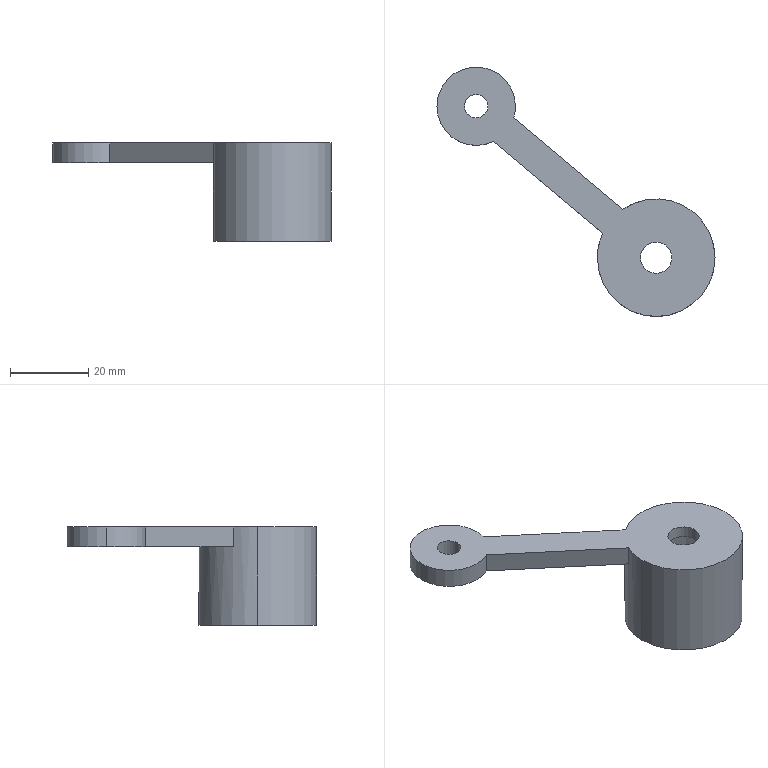Part | SolidWorks | features ICE 3, Extrusion 1 | 1 solid | 24 faces | box 70.91 x 63.63 x 25 mm | volume 8702 mm3 | cylinder 15 | plane 9 | commonest cylinder face diameters 2.5 x4 20 x3 6 x2 8 x2 26 x2 30 x2
STEP:
#1=CARTESIAN_POINT('',(56.492,-46.181,2.));
#2=VERTEX_POINT('',#1);
#3=CARTESIAN_POINT('',(55.918,-45.13,2.));
#4=VERTEX_POINT('',#3);
#5=CARTESIAN_POINT('',(57.168,-45.13,2.));
#6=DIRECTION('',(0.,0.,-1.));
#7=DIRECTION('',(-1.,0.,0.));
#8=AXIS2_PLACEMENT_3D('',#5,#6,#7);
#9=CIRCLE('',#8,1.25);
#10=EDGE_CURVE('',#2,#4,#9,.T.);
#11=ORIENTED_EDGE('',*,*,#10,.T.);
#12=CARTESIAN_POINT('',(55.918,-45.13,0.));
#13=VERTEX_POINT('',#12);
#14=CARTESIAN_POINT('',(55.918,-45.13,2.));
#15=DIRECTION('',(0.,0.,-1.));
#16=VECTOR('',#15,1000.);
#17=LINE('',#14,#16);
#18=EDGE_CURVE('',#4,#13,#17,.T.);
#19=ORIENTED_EDGE('',*,*,#18,.T.);
#20=CARTESIAN_POINT('',(56.492,-46.181,0.));
#21=VERTEX_POINT('',#20);
#22=CARTESIAN_POINT('',(57.168,-45.13,0.));
#23=DIRECTION('',(0.,0.,-1.));
#24=DIRECTION('',(-1.,0.,0.));
#25=AXIS2_PLACEMENT_3D('',#22,#23,#24);
#26=CIRCLE('',#25,1.25);
#27=EDGE_CURVE('',#21,#13,#26,.T.);
#28=ORIENTED_EDGE('',*,*,#27,.F.);
#29=CARTESIAN_POINT('',(56.492,-46.181,1.));
#30=DIRECTION('',(0.,0.,-1.));
#31=VECTOR('',#30,1000.);
#32=LINE('',#29,#31);
#33=EDGE_CURVE('',#2,#21,#32,.T.);
#34=ORIENTED_EDGE('',*,*,#33,.F.);
#35=EDGE_LOOP('',(#11,#19,#28,#34));
#36=FACE_OUTER_BOUND('',#35,.T.);
#37=CARTESIAN_POINT('',(57.168,-45.13,2.));
#38=DIRECTION('',(0.,0.,-1.));
#39=DIRECTION('',(-1.,0.,0.));
#40=AXIS2_PLACEMENT_3D('',#37,#38,#39);
#41=CYLINDRICAL_SURFACE('',#40,1.25);
#42=ADVANCED_FACE('',(#36),#41,.T.);
#43=CARTESIAN_POINT('',(58.91,-38.63,2.));
#44=VERTEX_POINT('',#43);
#45=CARTESIAN_POINT('',(57.74,-44.019,2.));
#46=VERTEX_POINT('',#45);
#47=CARTESIAN_POINT('',(45.91,-38.63,2.));
#48=DIRECTION('',(0.,0.,-1.));
#49=DIRECTION('',(-1.,0.,0.));
#50=AXIS2_PLACEMENT_3D('',#47,#48,#49);
#51=CIRCLE('',#50,13.);
#52=EDGE_CURVE('',#44,#46,#51,.T.);
#53=ORIENTED_EDGE('',*,*,#52,.F.);
#54=CARTESIAN_POINT('',(58.91,-38.63,-20.));
#55=VERTEX_POINT('',#54);
#56=CARTESIAN_POINT('',(58.91,-38.63,2.));
#57=DIRECTION('',(0.,0.,-1.));
#58=VECTOR('',#57,1000.);
#59=LINE('',#56,#58);
#60=EDGE_CURVE('',#44,#55,#59,.T.);
#61=ORIENTED_EDGE('',*,*,#60,.T.);
#62=CARTESIAN_POINT('',(32.91,-38.63,-20.));
#63=VERTEX_POINT('',#62);
#64=CARTESIAN_POINT('',(45.91,-38.63,-20.));
#65=DIRECTION('',(0.,0.,-1.));
#66=DIRECTION('',(-1.,0.,0.));
#67=AXIS2_PLACEMENT_3D('',#64,#65,#66);
#68=CIRCLE('',#67,13.);
#69=EDGE_CURVE('',#55,#63,#68,.T.);
#70=ORIENTED_EDGE('',*,*,#69,.T.);
#71=CARTESIAN_POINT('',(32.91,-38.63,2.));
#72=VERTEX_POINT('',#71);
#73=CARTESIAN_POINT('',(32.91,-38.63,2.));
#74=DIRECTION('',(0.,0.,-1.));
#75=VECTOR('',#74,1000.);
#76=LINE('',#73,#75);
#77=EDGE_CURVE('',#72,#63,#76,.T.);
#78=ORIENTED_EDGE('',*,*,#77,.F.);
#79=CARTESIAN_POINT('',(34.079,-44.019,2.));
#80=VERTEX_POINT('',#79);
#81=CARTESIAN_POINT('',(45.91,-38.63,2.));
#82=DIRECTION('',(0.,0.,-1.));
#83=DIRECTION('',(-1.,0.,0.));
#84=AXIS2_PLACEMENT_3D('',#81,#82,#83);
#85=CIRCLE('',#84,13.);
#86=EDGE_CURVE('',#80,#72,#85,.T.);
#87=ORIENTED_EDGE('',*,*,#86,.F.);
#88=CARTESIAN_POINT('',(34.079,-44.019,0.));
#89=VERTEX_POINT('',#88);
#90=CARTESIAN_POINT('',(34.079,-44.019,1.));
#91=DIRECTION('',(0.,0.,-1.));
#92=VECTOR('',#91,1000.);
#93=LINE('',#90,#92);
#94=EDGE_CURVE('',#80,#89,#93,.T.);
#95=ORIENTED_EDGE('',*,*,#94,.T.);
#96=CARTESIAN_POINT('',(35.328,-46.181,0.));
#97=VERTEX_POINT('',#96);
#98=CARTESIAN_POINT('',(45.91,-38.63,0.));
#99=DIRECTION('',(0.,0.,-1.));
#100=DIRECTION('',(-1.,0.,0.));
#101=AXIS2_PLACEMENT_3D('',#98,#99,#100);
#102=CIRCLE('',#101,13.);
#103=EDGE_CURVE('',#97,#89,#102,.T.);
#104=ORIENTED_EDGE('',*,*,#103,.F.);
#105=CARTESIAN_POINT('',(35.328,-46.181,2.));
#106=VERTEX_POINT('',#105);
#107=CARTESIAN_POINT('',(35.328,-46.181,1.));
#108=DIRECTION('',(0.,0.,1.));
#109=VECTOR('',#108,1000.);
#110=LINE('',#107,#109);
#111=EDGE_CURVE('',#97,#106,#110,.T.);
#112=ORIENTED_EDGE('',*,*,#111,.T.);
#113=CARTESIAN_POINT('',(45.91,-38.63,2.));
#114=DIRECTION('',(0.,0.,-1.));
#115=DIRECTION('',(-1.,0.,0.));
#116=AXIS2_PLACEMENT_3D('',#113,#114,#115);
#117=CIRCLE('',#116,13.);
#118=EDGE_CURVE('',#2,#106,#117,.T.);
#119=ORIENTED_EDGE('',*,*,#118,.F.);
#120=ORIENTED_EDGE('',*,*,#33,.T.);
#121=CARTESIAN_POINT('',(57.74,-44.019,0.));
#122=VERTEX_POINT('',#121);
#123=CARTESIAN_POINT('',(45.91,-38.63,0.));
#124=DIRECTION('',(0.,0.,-1.));
#125=DIRECTION('',(-1.,0.,0.));
#126=AXIS2_PLACEMENT_3D('',#123,#124,#125);
#127=CIRCLE('',#126,13.);
#128=EDGE_CURVE('',#122,#21,#127,.T.);
#129=ORIENTED_EDGE('',*,*,#128,.F.);
#130=CARTESIAN_POINT('',(57.74,-44.019,1.));
#131=DIRECTION('',(0.,0.,1.));
#132=VECTOR('',#131,1000.);
#133=LINE('',#130,#132);
#134=EDGE_CURVE('',#122,#46,#133,.T.);
#135=ORIENTED_EDGE('',*,*,#134,.T.);
#136=EDGE_LOOP('',(#53,#61,#70,#78,#87,#95,#104,#112,#119,#120,#129,#135));
#137=FACE_OUTER_BOUND('',#136,.T.);
#138=CARTESIAN_POINT('',(45.91,-38.63,2.));
#139=DIRECTION('',(0.,0.,-1.));
#140=DIRECTION('',(-1.,0.,0.));
#141=AXIS2_PLACEMENT_3D('',#138,#139,#140);
#142=CYLINDRICAL_SURFACE('',#141,13.);
#143=ADVANCED_FACE('',(#137),#142,.F.);
#144=CARTESIAN_POINT('',(-3.,0.,5.));
#145=VERTEX_POINT('',#144);
#146=CARTESIAN_POINT('',(3.,0.,5.));
#147=VERTEX_POINT('',#146);
#148=CARTESIAN_POINT('',(0.,0.,5.));
#149=DIRECTION('',(0.,0.,1.));
#150=DIRECTION('',(1.,0.,0.));
#151=AXIS2_PLACEMENT_3D('',#148,#149,#150);
#152=CIRCLE('',#151,3.);
#153=EDGE_CURVE('',#145,#147,#152,.T.);
#154=ORIENTED_EDGE('',*,*,#153,.T.);
#155=CARTESIAN_POINT('',(3.,0.,0.));
#156=VERTEX_POINT('',#155);
#157=CARTESIAN_POINT('',(3.,0.,5.));
#158=DIRECTION('',(0.,0.,-1.));
#159=VECTOR('',#158,1000.);
#160=LINE('',#157,#159);
#161=EDGE_CURVE('',#147,#156,#160,.T.);
#162=ORIENTED_EDGE('',*,*,#161,.T.);
#163=CARTESIAN_POINT('',(-3.,0.,0.));
#164=VERTEX_POINT('',#163);
#165=CARTESIAN_POINT('',(0.,0.,0.));
#166=DIRECTION('',(0.,0.,1.));
#167=DIRECTION('',(1.,0.,0.));
#168=AXIS2_PLACEMENT_3D('',#165,#166,#167);
#169=CIRCLE('',#168,3.);
#170=EDGE_CURVE('',#164,#156,#169,.T.);
#171=ORIENTED_EDGE('',*,*,#170,.F.);
#172=CARTESIAN_POINT('',(-3.,0.,5.));
#173=DIRECTION('',(0.,0.,-1.));
#174=VECTOR('',#173,1000.);
#175=LINE('',#172,#174);
#176=EDGE_CURVE('',#145,#164,#175,.T.);
#177=ORIENTED_EDGE('',*,*,#176,.F.);
#178=EDGE_LOOP('',(#154,#162,#171,#177));
#179=FACE_OUTER_BOUND('',#178,.T.);
#180=CARTESIAN_POINT('',(0.,0.,5.));
#181=DIRECTION('',(0.,0.,-1.));
#182=DIRECTION('',(-1.,0.,0.));
#183=AXIS2_PLACEMENT_3D('',#180,#181,#182);
#184=CYLINDRICAL_SURFACE('',#183,3.);
#185=ADVANCED_FACE('',(#179),#184,.F.);
#186=CARTESIAN_POINT('',(60.91,-38.63,5.));
#187=VERTEX_POINT('',#186);
#188=CARTESIAN_POINT('',(37.423,-26.262,5.));
#189=VERTEX_POINT('',#188);
#190=CARTESIAN_POINT('',(45.91,-38.63,5.));
#191=DIRECTION('',(0.,0.,1.));
#192=DIRECTION('',(1.,0.,0.));
#193=AXIS2_PLACEMENT_3D('',#190,#191,#192);
#194=CIRCLE('',#193,15.);
#195=EDGE_CURVE('',#187,#189,#194,.T.);
#196=ORIENTED_EDGE('',*,*,#195,.F.);
#197=CARTESIAN_POINT('',(60.91,-38.63,-20.));
#198=VERTEX_POINT('',#197);
#199=CARTESIAN_POINT('',(60.91,-38.63,5.));
#200=DIRECTION('',(0.,0.,-1.));
#201=VECTOR('',#200,1000.);
#202=LINE('',#199,#201);
#203=EDGE_CURVE('',#187,#198,#202,.T.);
#204=ORIENTED_EDGE('',*,*,#203,.T.);
#205=CARTESIAN_POINT('',(30.91,-38.63,-20.));
#206=VERTEX_POINT('',#205);
#207=CARTESIAN_POINT('',(45.91,-38.63,-20.));
#208=DIRECTION('',(0.,0.,-1.));
#209=DIRECTION('',(-1.,0.,0.));
#210=AXIS2_PLACEMENT_3D('',#207,#208,#209);
#211=CIRCLE('',#210,15.);
#212=EDGE_CURVE('',#206,#198,#211,.T.);
#213=ORIENTED_EDGE('',*,*,#212,.F.);
#214=CARTESIAN_POINT('',(30.91,-38.63,5.));
#215=VERTEX_POINT('',#214);
#216=CARTESIAN_POINT('',(30.91,-38.63,5.));
#217=DIRECTION('',(0.,0.,-1.));
#218=VECTOR('',#217,1000.);
#219=LINE('',#216,#218);
#220=EDGE_CURVE('',#215,#206,#219,.T.);
#221=ORIENTED_EDGE('',*,*,#220,.F.);
#222=CARTESIAN_POINT('',(32.273,-32.383,5.));
#223=VERTEX_POINT('',#222);
#224=CARTESIAN_POINT('',(45.91,-38.63,5.));
#225=DIRECTION('',(0.,0.,1.));
#226=DIRECTION('',(1.,0.,0.));
#227=AXIS2_PLACEMENT_3D('',#224,#225,#226);
#228=CIRCLE('',#227,15.);
#229=EDGE_CURVE('',#223,#215,#228,.T.);
#230=ORIENTED_EDGE('',*,*,#229,.F.);
#231=CARTESIAN_POINT('',(32.273,-32.383,0.));
#232=VERTEX_POINT('',#231);
#233=CARTESIAN_POINT('',(32.273,-32.383,5.));
#234=DIRECTION('',(0.,0.,-1.));
#235=VECTOR('',#234,1000.);
#236=LINE('',#233,#235);
#237=EDGE_CURVE('',#223,#232,#236,.T.);
#238=ORIENTED_EDGE('',*,*,#237,.T.);
#239=CARTESIAN_POINT('',(37.423,-26.262,0.));
#240=VERTEX_POINT('',#239);
#241=CARTESIAN_POINT('',(45.91,-38.63,0.));
#242=DIRECTION('',(0.,0.,-1.));
#243=DIRECTION('',(-1.,0.,0.));
#244=AXIS2_PLACEMENT_3D('',#241,#242,#243);
#245=CIRCLE('',#244,15.);
#246=EDGE_CURVE('',#232,#240,#245,.T.);
#247=ORIENTED_EDGE('',*,*,#246,.T.);
#248=CARTESIAN_POINT('',(37.423,-26.262,5.));
#249=DIRECTION('',(0.,0.,-1.));
#250=VECTOR('',#249,1000.);
#251=LINE('',#248,#250);
#252=EDGE_CURVE('',#189,#240,#251,.T.);
#253=ORIENTED_EDGE('',*,*,#252,.F.);
#254=EDGE_LOOP('',(#196,#204,#213,#221,#230,#238,#247,#253));
#255=FACE_OUTER_BOUND('',#254,.T.);
#256=CARTESIAN_POINT('',(45.91,-38.63,5.));
#257=DIRECTION('',(0.,0.,-1.));
#258=DIRECTION('',(-1.,0.,0.));
#259=AXIS2_PLACEMENT_3D('',#256,#257,#258);
#260=CYLINDRICAL_SURFACE('',#259,15.);
#261=ADVANCED_FACE('',(#255),#260,.T.);
#262=CARTESIAN_POINT('',(10.,0.,5.));
#263=VERTEX_POINT('',#262);
#264=CARTESIAN_POINT('',(-10.,0.,5.));
#265=VERTEX_POINT('',#264);
#266=CARTESIAN_POINT('',(0.,0.,5.));
#267=DIRECTION('',(0.,0.,1.));
#268=DIRECTION('',(1.,0.,0.));
#269=AXIS2_PLACEMENT_3D('',#266,#267,#268);
#270=CIRCLE('',#269,10.);
#271=EDGE_CURVE('',#263,#265,#270,.T.);
#272=ORIENTED_EDGE('',*,*,#271,.F.);
#273=CARTESIAN_POINT('',(10.,0.,0.));
#274=VERTEX_POINT('',#273);
#275=CARTESIAN_POINT('',(10.,0.,5.));
#276=DIRECTION('',(0.,0.,-1.));
#277=VECTOR('',#276,1000.);
#278=LINE('',#275,#277);
#279=EDGE_CURVE('',#263,#274,#278,.T.);
#280=ORIENTED_EDGE('',*,*,#279,.T.);
#281=CARTESIAN_POINT('',(-10.,0.,0.));
#282=VERTEX_POINT('',#281);
#283=CARTESIAN_POINT('',(0.,0.,0.));
#284=DIRECTION('',(0.,0.,1.));
#285=DIRECTION('',(1.,0.,0.));
#286=AXIS2_PLACEMENT_3D('',#283,#284,#285);
#287=CIRCLE('',#286,10.);
#288=EDGE_CURVE('',#274,#282,#287,.T.);
#289=ORIENTED_EDGE('',*,*,#288,.T.);
#290=CARTESIAN_POINT('',(-10.,0.,5.));
#291=DIRECTION('',(0.,0.,-1.));
#292=VECTOR('',#291,1000.);
#293=LINE('',#290,#292);
#294=EDGE_CURVE('',#265,#282,#293,.T.);
#295=ORIENTED_EDGE('',*,*,#294,.F.);
#296=EDGE_LOOP('',(#272,#280,#289,#295));
#297=FACE_OUTER_BOUND('',#296,.T.);
#298=CARTESIAN_POINT('',(0.,0.,5.));
#299=DIRECTION('',(0.,0.,-1.));
#300=DIRECTION('',(-1.,0.,0.));
#301=AXIS2_PLACEMENT_3D('',#298,#299,#300);
#302=CYLINDRICAL_SURFACE('',#301,10.);
#303=ADVANCED_FACE('',(#297),#302,.T.);
#304=CARTESIAN_POINT('',(4.438,-8.961,5.));
#305=VERTEX_POINT('',#304);
#306=CARTESIAN_POINT('',(0.,0.,5.));
#307=DIRECTION('',(0.,0.,1.));
#308=DIRECTION('',(1.,0.,0.));
#309=AXIS2_PLACEMENT_3D('',#306,#307,#308);
#310=CIRCLE('',#309,10.);
#311=EDGE_CURVE('',#265,#305,#310,.T.);
#312=ORIENTED_EDGE('',*,*,#311,.F.);
#313=ORIENTED_EDGE('',*,*,#294,.T.);
#314=CARTESIAN_POINT('',(4.438,-8.961,0.));
#315=VERTEX_POINT('',#314);
#316=CARTESIAN_POINT('',(0.,0.,0.));
#317=DIRECTION('',(0.,0.,1.));
#318=DIRECTION('',(1.,0.,0.));
#319=AXIS2_PLACEMENT_3D('',#316,#317,#318);
#320=CIRCLE('',#319,10.);
#321=EDGE_CURVE('',#282,#315,#320,.T.);
#322=ORIENTED_EDGE('',*,*,#321,.T.);
#323=CARTESIAN_POINT('',(4.438,-8.961,5.));
#324=DIRECTION('',(0.,0.,-1.));
#325=VECTOR('',#324,1000.);
#326=LINE('',#323,#325);
#327=EDGE_CURVE('',#305,#315,#326,.T.);
#328=ORIENTED_EDGE('',*,*,#327,.F.);
#329=EDGE_LOOP('',(#312,#313,#322,#328));
#330=FACE_OUTER_BOUND('',#329,.T.);
#331=CARTESIAN_POINT('',(0.,0.,5.));
#332=DIRECTION('',(0.,0.,-1.));
#333=DIRECTION('',(-1.,0.,0.));
#334=AXIS2_PLACEMENT_3D('',#331,#332,#333);
#335=CYLINDRICAL_SURFACE('',#334,10.);
#336=ADVANCED_FACE('',(#330),#335,.T.);
#337=CARTESIAN_POINT('',(41.91,-38.63,5.));
#338=VERTEX_POINT('',#337);
#339=CARTESIAN_POINT('',(49.91,-38.63,5.));
#340=VERTEX_POINT('',#339);
#341=CARTESIAN_POINT('',(45.91,-38.63,5.));
#342=DIRECTION('',(0.,0.,1.));
#343=DIRECTION('',(1.,0.,0.));
#344=AXIS2_PLACEMENT_3D('',#341,#342,#343);
#345=CIRCLE('',#344,4.);
#346=EDGE_CURVE('',#338,#340,#345,.T.);
#347=ORIENTED_EDGE('',*,*,#346,.T.);
#348=CARTESIAN_POINT('',(49.91,-38.63,2.));
#349=VERTEX_POINT('',#348);
#350=CARTESIAN_POINT('',(49.91,-38.63,5.));
#351=DIRECTION('',(0.,0.,-1.));
#352=VECTOR('',#351,1000.);
#353=LINE('',#350,#352);
#354=EDGE_CURVE('',#340,#349,#353,.T.);
#355=ORIENTED_EDGE('',*,*,#354,.T.);
#356=CARTESIAN_POINT('',(41.91,-38.63,2.));
#357=VERTEX_POINT('',#356);
#358=CARTESIAN_POINT('',(45.91,-38.63,2.));
#359=DIRECTION('',(0.,0.,-1.));
#360=DIRECTION('',(-1.,0.,0.));
#361=AXIS2_PLACEMENT_3D('',#358,#359,#360);
#362=CIRCLE('',#361,4.);
#363=EDGE_CURVE('',#349,#357,#362,.T.);
#364=ORIENTED_EDGE('',*,*,#363,.T.);
#365=CARTESIAN_POINT('',(41.91,-38.63,5.));
#366=DIRECTION('',(0.,0.,-1.));
#367=VECTOR('',#366,1000.);
#368=LINE('',#365,#367);
#369=EDGE_CURVE('',#338,#357,#368,.T.);
#370=ORIENTED_EDGE('',*,*,#369,.F.);
#371=EDGE_LOOP('',(#347,#355,#364,#370));
#372=FACE_OUTER_BOUND('',#371,.T.);
#373=CARTESIAN_POINT('',(45.91,-38.63,5.));
#374=DIRECTION('',(0.,0.,-1.));
#375=DIRECTION('',(-1.,0.,0.));
#376=AXIS2_PLACEMENT_3D('',#373,#374,#375);
#377=CYLINDRICAL_SURFACE('',#376,4.);
#378=ADVANCED_FACE('',(#372),#377,.F.);
#379=ORIENTED_EDGE('',*,*,#170,.T.);
#380=CARTESIAN_POINT('',(0.,0.,0.));
#381=DIRECTION('',(0.,0.,1.));
#382=DIRECTION('',(1.,0.,0.));
#383=AXIS2_PLACEMENT_3D('',#380,#381,#382);
#384=CIRCLE('',#383,3.);
#385=EDGE_CURVE('',#156,#164,#384,.T.);
#386=ORIENTED_EDGE('',*,*,#385,.T.);
#387=EDGE_LOOP('',(#379,#386));
#388=FACE_BOUND('',#387,.T.);
#389=ORIENTED_EDGE('',*,*,#246,.F.);
#390=CARTESIAN_POINT('',(4.438,-8.961,0.));
#391=DIRECTION('',(0.7652,-0.6438,0.));
#392=VECTOR('',#391,1000.);
#393=LINE('',#390,#392);
#394=EDGE_CURVE('',#315,#232,#393,.T.);
#395=ORIENTED_EDGE('',*,*,#394,.F.);
#396=ORIENTED_EDGE('',*,*,#321,.F.);
#397=ORIENTED_EDGE('',*,*,#288,.F.);
#398=CARTESIAN_POINT('',(9.588,-2.84,0.));
#399=VERTEX_POINT('',#398);
#400=CARTESIAN_POINT('',(0.,0.,0.));
#401=DIRECTION('',(0.,0.,1.));
#402=DIRECTION('',(1.,0.,0.));
#403=AXIS2_PLACEMENT_3D('',#400,#401,#402);
#404=CIRCLE('',#403,10.);
#405=EDGE_CURVE('',#399,#274,#404,.T.);
#406=ORIENTED_EDGE('',*,*,#405,.F.);
#407=CARTESIAN_POINT('',(9.588,-2.84,0.));
#408=DIRECTION('',(-0.7652,0.6438,0.));
#409=VECTOR('',#408,1000.);
#410=LINE('',#407,#409);
#411=EDGE_CURVE('',#240,#399,#410,.T.);
#412=ORIENTED_EDGE('',*,*,#411,.F.);
#413=EDGE_LOOP('',(#389,#395,#396,#397,#406,#412));
#414=FACE_OUTER_BOUND('',#413,.T.);
#415=CARTESIAN_POINT('',(0.,0.,0.));
#416=DIRECTION('',(0.,0.,1.));
#417=DIRECTION('',(1.,0.,0.));
#418=AXIS2_PLACEMENT_3D('',#415,#416,#417);
#419=PLANE('',#418);
#420=ADVANCED_FACE('',(#388,#414),#419,.F.);
#421=CARTESIAN_POINT('',(47.158,-25.69,0.));
#422=VERTEX_POINT('',#421);
#423=CARTESIAN_POINT('',(44.661,-25.69,0.));
#424=VERTEX_POINT('',#423);
#425=CARTESIAN_POINT('',(45.91,-25.63,0.));
#426=DIRECTION('',(0.,0.,-1.));
#427=DIRECTION('',(-1.,0.,0.));
#428=AXIS2_PLACEMENT_3D('',#425,#426,#427);
#429=CIRCLE('',#428,1.25);
#430=EDGE_CURVE('',#422,#424,#429,.T.);
#431=ORIENTED_EDGE('',*,*,#430,.T.);
#432=CARTESIAN_POINT('',(45.91,-38.63,0.));
#433=DIRECTION('',(0.,0.,-1.));
#434=DIRECTION('',(-1.,0.,0.));
#435=AXIS2_PLACEMENT_3D('',#432,#433,#434);
#436=CIRCLE('',#435,13.);
#437=EDGE_CURVE('',#424,#422,#436,.T.);
#438=ORIENTED_EDGE('',*,*,#437,.T.);
#439=EDGE_LOOP('',(#431,#438));
#440=FACE_OUTER_BOUND('',#439,.T.);
#441=CARTESIAN_POINT('',(0.,0.,0.));
#442=DIRECTION('',(0.,0.,1.));
#443=DIRECTION('',(1.,0.,0.));
#444=AXIS2_PLACEMENT_3D('',#441,#442,#443);
#445=PLANE('',#444);
#446=ADVANCED_FACE('',(#440),#445,.F.);
#447=ORIENTED_EDGE('',*,*,#27,.T.);
#448=CARTESIAN_POINT('',(57.168,-45.13,0.));
#449=DIRECTION('',(0.,0.,-1.));
#450=DIRECTION('',(-1.,0.,0.));
#451=AXIS2_PLACEMENT_3D('',#448,#449,#450);
#452=CIRCLE('',#451,1.25);
#453=EDGE_CURVE('',#13,#122,#452,.T.);
#454=ORIENTED_EDGE('',*,*,#453,.T.);
#455=ORIENTED_EDGE('',*,*,#128,.T.);
#456=EDGE_LOOP('',(#447,#454,#455));
#457=FACE_OUTER_BOUND('',#456,.T.);
#458=CARTESIAN_POINT('',(0.,0.,0.));
#459=DIRECTION('',(0.,0.,1.));
#460=DIRECTION('',(1.,0.,0.));
#461=AXIS2_PLACEMENT_3D('',#458,#459,#460);
#462=PLANE('',#461);
#463=ADVANCED_FACE('',(#457),#462,.F.);
#464=ORIENTED_EDGE('',*,*,#354,.F.);
#465=CARTESIAN_POINT('',(45.91,-38.63,5.));
#466=DIRECTION('',(0.,0.,1.));
#467=DIRECTION('',(1.,0.,0.));
#468=AXIS2_PLACEMENT_3D('',#465,#466,#467);
#469=CIRCLE('',#468,4.);
#470=EDGE_CURVE('',#340,#338,#469,.T.);
#471=ORIENTED_EDGE('',*,*,#470,.T.);
#472=ORIENTED_EDGE('',*,*,#369,.T.);
#473=CARTESIAN_POINT('',(45.91,-38.63,2.));
#474=DIRECTION('',(0.,0.,-1.));
#475=DIRECTION('',(-1.,0.,0.));
#476=AXIS2_PLACEMENT_3D('',#473,#474,#475);
#477=CIRCLE('',#476,4.);
#478=EDGE_CURVE('',#357,#349,#477,.T.);
#479=ORIENTED_EDGE('',*,*,#478,.T.);
#480=EDGE_LOOP('',(#464,#471,#472,#479));
#481=FACE_OUTER_BOUND('',#480,.T.);
#482=CARTESIAN_POINT('',(45.91,-38.63,5.));
#483=DIRECTION('',(0.,0.,-1.));
#484=DIRECTION('',(-1.,0.,0.));
#485=AXIS2_PLACEMENT_3D('',#482,#483,#484);
#486=CYLINDRICAL_SURFACE('',#485,4.);
#487=ADVANCED_FACE('',(#481),#486,.F.);
#488=ORIENTED_EDGE('',*,*,#153,.F.);
#489=CARTESIAN_POINT('',(0.,0.,5.));
#490=DIRECTION('',(0.,0.,1.));
#491=DIRECTION('',(1.,0.,0.));
#492=AXIS2_PLACEMENT_3D('',#489,#490,#491);
#493=CIRCLE('',#492,3.);
#494=EDGE_CURVE('',#147,#145,#493,.T.);
#495=ORIENTED_EDGE('',*,*,#494,.F.);
#496=EDGE_LOOP('',(#488,#495));
#497=FACE_BOUND('',#496,.T.);
#498=CARTESIAN_POINT('',(9.588,-2.84,5.));
#499=VERTEX_POINT('',#498);
#500=CARTESIAN_POINT('',(0.,0.,5.));
#501=DIRECTION('',(0.,0.,1.));
#502=DIRECTION('',(1.,0.,0.));
#503=AXIS2_PLACEMENT_3D('',#500,#501,#502);
#504=CIRCLE('',#503,10.);
#505=EDGE_CURVE('',#499,#263,#504,.T.);
#506=ORIENTED_EDGE('',*,*,#505,.T.);
#507=ORIENTED_EDGE('',*,*,#271,.T.);
#508=ORIENTED_EDGE('',*,*,#311,.T.);
#509=CARTESIAN_POINT('',(4.438,-8.961,5.));
#510=DIRECTION('',(0.7652,-0.6438,0.));
#511=VECTOR('',#510,1000.);
#512=LINE('',#509,#511);
#513=EDGE_CURVE('',#305,#223,#512,.T.);
#514=ORIENTED_EDGE('',*,*,#513,.T.);
#515=ORIENTED_EDGE('',*,*,#229,.T.);
#516=CARTESIAN_POINT('',(45.91,-38.63,5.));
#517=DIRECTION('',(0.,0.,1.));
#518=DIRECTION('',(1.,0.,0.));
#519=AXIS2_PLACEMENT_3D('',#516,#517,#518);
#520=CIRCLE('',#519,15.);
#521=EDGE_CURVE('',#215,#187,#520,.T.);
#522=ORIENTED_EDGE('',*,*,#521,.T.);
#523=ORIENTED_EDGE('',*,*,#195,.T.);
#524=CARTESIAN_POINT('',(9.588,-2.84,5.));
#525=DIRECTION('',(-0.7652,0.6438,0.));
#526=VECTOR('',#525,1000.);
#527=LINE('',#524,#526);
#528=EDGE_CURVE('',#189,#499,#527,.T.);
#529=ORIENTED_EDGE('',*,*,#528,.T.);
#530=EDGE_LOOP('',(#506,#507,#508,#514,#515,#522,#523,#529));
#531=FACE_OUTER_BOUND('',#530,.T.);
#532=ORIENTED_EDGE('',*,*,#346,.F.);
#533=ORIENTED_EDGE('',*,*,#470,.F.);
#534=EDGE_LOOP('',(#532,#533));
#535=FACE_BOUND('',#534,.T.);
#536=CARTESIAN_POINT('',(0.,0.,5.));
#537=DIRECTION('',(0.,0.,1.));
#538=DIRECTION('',(1.,0.,0.));
#539=AXIS2_PLACEMENT_3D('',#536,#537,#538);
#540=PLANE('',#539);
#541=ADVANCED_FACE('',(#497,#531,#535),#540,.T.);
#542=CARTESIAN_POINT('',(34.652,-45.13,0.));
#543=DIRECTION('',(0.,0.,-1.));
#544=DIRECTION('',(-1.,0.,0.));
#545=AXIS2_PLACEMENT_3D('',#542,#543,#544);
#546=CIRCLE('',#545,1.25);
#547=EDGE_CURVE('',#89,#97,#546,.T.);
#548=ORIENTED_EDGE('',*,*,#547,.T.);
#549=ORIENTED_EDGE('',*,*,#103,.T.);
#550=EDGE_LOOP('',(#548,#549));
#551=FACE_OUTER_BOUND('',#550,.T.);
#552=CARTESIAN_POINT('',(0.,0.,0.));
#553=DIRECTION('',(0.,0.,1.));
#554=DIRECTION('',(1.,0.,0.));
#555=AXIS2_PLACEMENT_3D('',#552,#553,#554);
#556=PLANE('',#555);
#557=ADVANCED_FACE('',(#551),#556,.F.);
#558=ORIENTED_EDGE('',*,*,#279,.F.);
#559=ORIENTED_EDGE('',*,*,#505,.F.);
#560=CARTESIAN_POINT('',(9.588,-2.84,5.));
#561=DIRECTION('',(0.,0.,-1.));
#562=VECTOR('',#561,1000.);
#563=LINE('',#560,#562);
#564=EDGE_CURVE('',#499,#399,#563,.T.);
#565=ORIENTED_EDGE('',*,*,#564,.T.);
#566=ORIENTED_EDGE('',*,*,#405,.T.);
#567=EDGE_LOOP('',(#558,#559,#565,#566));
#568=FACE_OUTER_BOUND('',#567,.T.);
#569=CARTESIAN_POINT('',(0.,0.,5.));
#570=DIRECTION('',(0.,0.,-1.));
#571=DIRECTION('',(-1.,0.,0.));
#572=AXIS2_PLACEMENT_3D('',#569,#570,#571);
#573=CYLINDRICAL_SURFACE('',#572,10.);
#574=ADVANCED_FACE('',(#568),#573,.T.);
#575=ORIENTED_EDGE('',*,*,#394,.T.);
#576=ORIENTED_EDGE('',*,*,#237,.F.);
#577=ORIENTED_EDGE('',*,*,#513,.F.);
#578=ORIENTED_EDGE('',*,*,#327,.T.);
#579=EDGE_LOOP('',(#575,#576,#577,#578));
#580=FACE_OUTER_BOUND('',#579,.T.);
#581=CARTESIAN_POINT('',(4.438,-8.961,5.));
#582=DIRECTION('',(0.6438,0.7652,0.));
#583=DIRECTION('',(-0.7652,0.6438,0.));
#584=AXIS2_PLACEMENT_3D('',#581,#582,#583);
#585=PLANE('',#584);
#586=ADVANCED_FACE('',(#580),#585,.F.);
#587=ORIENTED_EDGE('',*,*,#203,.F.);
#588=ORIENTED_EDGE('',*,*,#521,.F.);
#589=ORIENTED_EDGE('',*,*,#220,.T.);
#590=CARTESIAN_POINT('',(45.91,-38.63,-20.));
#591=DIRECTION('',(0.,0.,-1.));
#592=DIRECTION('',(-1.,0.,0.));
#593=AXIS2_PLACEMENT_3D('',#590,#591,#592);
#594=CIRCLE('',#593,15.);
#595=EDGE_CURVE('',#198,#206,#594,.T.);
#596=ORIENTED_EDGE('',*,*,#595,.F.);
#597=EDGE_LOOP('',(#587,#588,#589,#596));
#598=FACE_OUTER_BOUND('',#597,.T.);
#599=CARTESIAN_POINT('',(45.91,-38.63,5.));
#600=DIRECTION('',(0.,0.,-1.));
#601=DIRECTION('',(-1.,0.,0.));
#602=AXIS2_PLACEMENT_3D('',#599,#600,#601);
#603=CYLINDRICAL_SURFACE('',#602,15.);
#604=ADVANCED_FACE('',(#598),#603,.T.);
#605=ORIENTED_EDGE('',*,*,#411,.T.);
#606=ORIENTED_EDGE('',*,*,#564,.F.);
#607=ORIENTED_EDGE('',*,*,#528,.F.);
#608=ORIENTED_EDGE('',*,*,#252,.T.);
#609=EDGE_LOOP('',(#605,#606,#607,#608));
#610=FACE_OUTER_BOUND('',#609,.T.);
#611=CARTESIAN_POINT('',(9.588,-2.84,5.));
#612=DIRECTION('',(-0.6438,-0.7652,0.));
#613=DIRECTION('',(0.7652,-0.6438,0.));
#614=AXIS2_PLACEMENT_3D('',#611,#612,#613);
#615=PLANE('',#614);
#616=ADVANCED_FACE('',(#610),#615,.F.);
#617=ORIENTED_EDGE('',*,*,#161,.F.);
#618=ORIENTED_EDGE('',*,*,#494,.T.);
#619=ORIENTED_EDGE('',*,*,#176,.T.);
#620=ORIENTED_EDGE('',*,*,#385,.F.);
#621=EDGE_LOOP('',(#617,#618,#619,#620));
#622=FACE_OUTER_BOUND('',#621,.T.);
#623=CARTESIAN_POINT('',(0.,0.,5.));
#624=DIRECTION('',(0.,0.,-1.));
#625=DIRECTION('',(-1.,0.,0.));
#626=AXIS2_PLACEMENT_3D('',#623,#624,#625);
#627=CYLINDRICAL_SURFACE('',#626,3.);
#628=ADVANCED_FACE('',(#622),#627,.F.);
#629=ORIENTED_EDGE('',*,*,#60,.F.);
#630=CARTESIAN_POINT('',(47.158,-25.69,2.));
#631=VERTEX_POINT('',#630);
#632=CARTESIAN_POINT('',(45.91,-38.63,2.));
#633=DIRECTION('',(0.,0.,-1.));
#634=DIRECTION('',(-1.,0.,0.));
#635=AXIS2_PLACEMENT_3D('',#632,#633,#634);
#636=CIRCLE('',#635,13.);
#637=EDGE_CURVE('',#631,#44,#636,.T.);
#638=ORIENTED_EDGE('',*,*,#637,.F.);
#639=CARTESIAN_POINT('',(47.158,-25.69,1.));
#640=DIRECTION('',(0.,0.,-1.));
#641=VECTOR('',#640,1000.);
#642=LINE('',#639,#641);
#643=EDGE_CURVE('',#631,#422,#642,.T.);
#644=ORIENTED_EDGE('',*,*,#643,.T.);
#645=ORIENTED_EDGE('',*,*,#437,.F.);
#646=CARTESIAN_POINT('',(44.661,-25.69,2.));
#647=VERTEX_POINT('',#646);
#648=CARTESIAN_POINT('',(44.661,-25.69,1.));
#649=DIRECTION('',(0.,0.,1.));
#650=VECTOR('',#649,1000.);
#651=LINE('',#648,#650);
#652=EDGE_CURVE('',#424,#647,#651,.T.);
#653=ORIENTED_EDGE('',*,*,#652,.T.);
#654=CARTESIAN_POINT('',(45.91,-38.63,2.));
#655=DIRECTION('',(0.,0.,-1.));
#656=DIRECTION('',(-1.,0.,0.));
#657=AXIS2_PLACEMENT_3D('',#654,#655,#656);
#658=CIRCLE('',#657,13.);
#659=EDGE_CURVE('',#72,#647,#658,.T.);
#660=ORIENTED_EDGE('',*,*,#659,.F.);
#661=ORIENTED_EDGE('',*,*,#77,.T.);
#662=CARTESIAN_POINT('',(45.91,-38.63,-20.));
#663=DIRECTION('',(0.,0.,-1.));
#664=DIRECTION('',(-1.,0.,0.));
#665=AXIS2_PLACEMENT_3D('',#662,#663,#664);
#666=CIRCLE('',#665,13.);
#667=EDGE_CURVE('',#63,#55,#666,.T.);
#668=ORIENTED_EDGE('',*,*,#667,.T.);
#669=EDGE_LOOP('',(#629,#638,#644,#645,#653,#660,#661,#668));
#670=FACE_OUTER_BOUND('',#669,.T.);
#671=CARTESIAN_POINT('',(45.91,-38.63,2.));
#672=DIRECTION('',(0.,0.,-1.));
#673=DIRECTION('',(-1.,0.,0.));
#674=AXIS2_PLACEMENT_3D('',#671,#672,#673);
#675=CYLINDRICAL_SURFACE('',#674,13.);
#676=ADVANCED_FACE('',(#670),#675,.F.);
#677=CARTESIAN_POINT('',(34.652,-45.13,2.));
#678=DIRECTION('',(0.,0.,-1.));
#679=DIRECTION('',(-1.,0.,0.));
#680=AXIS2_PLACEMENT_3D('',#677,#678,#679);
#681=CIRCLE('',#680,1.25);
#682=EDGE_CURVE('',#80,#106,#681,.T.);
#683=ORIENTED_EDGE('',*,*,#682,.F.);
#684=ORIENTED_EDGE('',*,*,#86,.T.);
#685=ORIENTED_EDGE('',*,*,#659,.T.);
#686=CARTESIAN_POINT('',(45.91,-25.63,2.));
#687=DIRECTION('',(0.,0.,-1.));
#688=DIRECTION('',(-1.,0.,0.));
#689=AXIS2_PLACEMENT_3D('',#686,#687,#688);
#690=CIRCLE('',#689,1.25);
#691=EDGE_CURVE('',#631,#647,#690,.T.);
#692=ORIENTED_EDGE('',*,*,#691,.F.);
#693=ORIENTED_EDGE('',*,*,#637,.T.);
#694=ORIENTED_EDGE('',*,*,#52,.T.);
#695=CARTESIAN_POINT('',(57.168,-45.13,2.));
#696=DIRECTION('',(0.,0.,-1.));
#697=DIRECTION('',(-1.,0.,0.));
#698=AXIS2_PLACEMENT_3D('',#695,#696,#697);
#699=CIRCLE('',#698,1.25);
#700=EDGE_CURVE('',#4,#46,#699,.T.);
#701=ORIENTED_EDGE('',*,*,#700,.F.);
#702=ORIENTED_EDGE('',*,*,#10,.F.);
#703=ORIENTED_EDGE('',*,*,#118,.T.);
#704=EDGE_LOOP('',(#683,#684,#685,#692,#693,#694,#701,#702,#703));
#705=FACE_OUTER_BOUND('',#704,.T.);
#706=ORIENTED_EDGE('',*,*,#478,.F.);
#707=ORIENTED_EDGE('',*,*,#363,.F.);
#708=EDGE_LOOP('',(#706,#707));
#709=FACE_BOUND('',#708,.T.);
#710=CARTESIAN_POINT('',(45.91,-38.63,2.));
#711=DIRECTION('',(0.,0.,-1.));
#712=DIRECTION('',(-1.,0.,0.));
#713=AXIS2_PLACEMENT_3D('',#710,#711,#712);
#714=PLANE('',#713);
#715=ADVANCED_FACE('',(#705,#709),#714,.T.);
#716=ORIENTED_EDGE('',*,*,#643,.F.);
#717=ORIENTED_EDGE('',*,*,#691,.T.);
#718=ORIENTED_EDGE('',*,*,#652,.F.);
#719=ORIENTED_EDGE('',*,*,#430,.F.);
#720=EDGE_LOOP('',(#716,#717,#718,#719));
#721=FACE_OUTER_BOUND('',#720,.T.);
#722=CARTESIAN_POINT('',(45.91,-25.63,2.));
#723=DIRECTION('',(0.,0.,-1.));
#724=DIRECTION('',(-1.,0.,0.));
#725=AXIS2_PLACEMENT_3D('',#722,#723,#724);
#726=CYLINDRICAL_SURFACE('',#725,1.25);
#727=ADVANCED_FACE('',(#721),#726,.T.);
#728=ORIENTED_EDGE('',*,*,#18,.F.);
#729=ORIENTED_EDGE('',*,*,#700,.T.);
#730=ORIENTED_EDGE('',*,*,#134,.F.);
#731=ORIENTED_EDGE('',*,*,#453,.F.);
#732=EDGE_LOOP('',(#728,#729,#730,#731));
#733=FACE_OUTER_BOUND('',#732,.T.);
#734=CARTESIAN_POINT('',(57.168,-45.13,2.));
#735=DIRECTION('',(0.,0.,-1.));
#736=DIRECTION('',(-1.,0.,0.));
#737=AXIS2_PLACEMENT_3D('',#734,#735,#736);
#738=CYLINDRICAL_SURFACE('',#737,1.25);
#739=ADVANCED_FACE('',(#733),#738,.T.);
#740=ORIENTED_EDGE('',*,*,#94,.F.);
#741=ORIENTED_EDGE('',*,*,#682,.T.);
#742=ORIENTED_EDGE('',*,*,#111,.F.);
#743=ORIENTED_EDGE('',*,*,#547,.F.);
#744=EDGE_LOOP('',(#740,#741,#742,#743));
#745=FACE_OUTER_BOUND('',#744,.T.);
#746=CARTESIAN_POINT('',(34.652,-45.13,2.));
#747=DIRECTION('',(0.,0.,-1.));
#748=DIRECTION('',(-1.,0.,0.));
#749=AXIS2_PLACEMENT_3D('',#746,#747,#748);
#750=CYLINDRICAL_SURFACE('',#749,1.25);
#751=ADVANCED_FACE('',(#745),#750,.T.);
#752=ORIENTED_EDGE('',*,*,#212,.T.);
#753=ORIENTED_EDGE('',*,*,#595,.T.);
#754=EDGE_LOOP('',(#752,#753));
#755=FACE_OUTER_BOUND('',#754,.T.);
#756=ORIENTED_EDGE('',*,*,#667,.F.);
#757=ORIENTED_EDGE('',*,*,#69,.F.);
#758=EDGE_LOOP('',(#756,#757));
#759=FACE_BOUND('',#758,.T.);
#760=CARTESIAN_POINT('',(45.91,-38.63,-20.));
#761=DIRECTION('',(0.,0.,-1.));
#762=DIRECTION('',(-1.,0.,0.));
#763=AXIS2_PLACEMENT_3D('',#760,#761,#762);
#764=PLANE('',#763);
#765=ADVANCED_FACE('',(#755,#759),#764,.T.);
#766=CLOSED_SHELL('',(#42,#143,#185,#261,#303,#336,#378,#420,#446,#463,#487,#541,#557,#574,#586,#604,#616,#628,#676,#715,#727,#739,#751,#765));
#767=MANIFOLD_SOLID_BREP('',#766);
#768=CARTESIAN_POINT('',(0.,0.,0.));
#769=DIRECTION('',(0.,0.,1.));
#770=DIRECTION('',(1.,0.,0.));
#771=AXIS2_PLACEMENT_3D('',#768,#769,#770);
#772=(LENGTH_UNIT()NAMED_UNIT(*)SI_UNIT(.MILLI.,.METRE.));
#773=UNCERTAINTY_MEASURE_WITH_UNIT(LENGTH_MEASURE(0.00001),#772,'','');
#774=(NAMED_UNIT(*)PLANE_ANGLE_UNIT()SI_UNIT($,.RADIAN.));
#775=(NAMED_UNIT(*)SI_UNIT($,.STERADIAN.)SOLID_ANGLE_UNIT());
#776=(GEOMETRIC_REPRESENTATION_CONTEXT(3)GLOBAL_UNCERTAINTY_ASSIGNED_CONTEXT((#773))GLOBAL_UNIT_ASSIGNED_CONTEXT((#772,#774,#775))REPRESENTATION_CONTEXT('',''));
#777=ADVANCED_BREP_SHAPE_REPRESENTATION('',(#767,#771),#776);